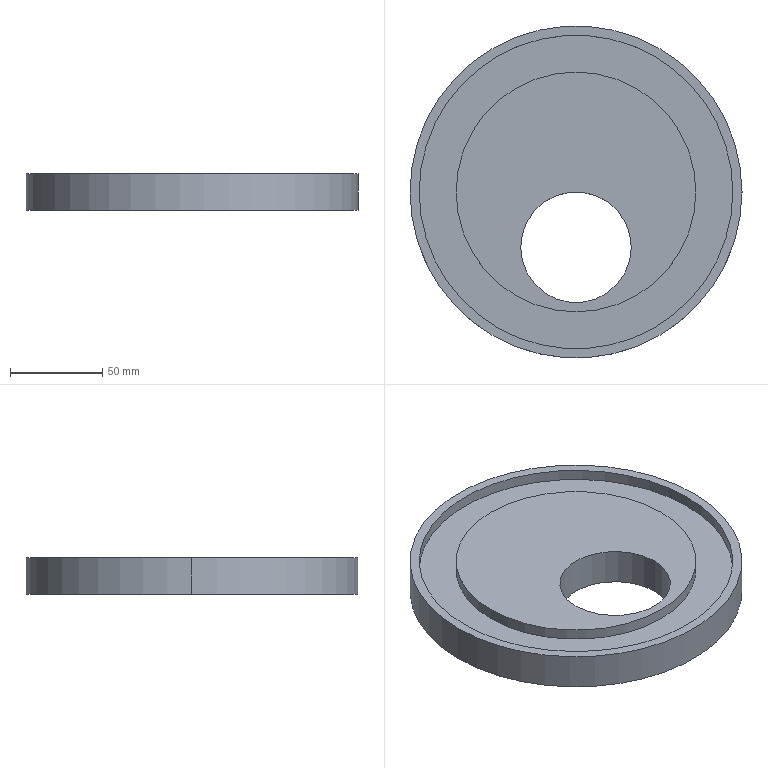Part | SolidWorks | features ICE 2, Extrusion 1 | 1 solid | 18 faces | box 180 x 180 x 20 mm | volume 339292 mm3 | cylinder 12 | plane 6 | commonest cylinder face diameters 130 x4 170 x4 60 x2 180 x2
STEP:
#1=CARTESIAN_POINT('',(-65.,30.,6.));
#2=VERTEX_POINT('',#1);
#3=CARTESIAN_POINT('',(65.,30.,6.));
#4=VERTEX_POINT('',#3);
#5=CARTESIAN_POINT('',(0.,30.,6.));
#6=DIRECTION('',(0.,0.,-1.));
#7=DIRECTION('',(-1.,0.,0.));
#8=AXIS2_PLACEMENT_3D('',#5,#6,#7);
#9=CIRCLE('',#8,65.);
#10=EDGE_CURVE('',#2,#4,#9,.T.);
#11=ORIENTED_EDGE('',*,*,#10,.T.);
#12=CARTESIAN_POINT('',(65.,30.,0.));
#13=VERTEX_POINT('',#12);
#14=CARTESIAN_POINT('',(65.,30.,6.));
#15=DIRECTION('',(0.,0.,-1.));
#16=VECTOR('',#15,1000.);
#17=LINE('',#14,#16);
#18=EDGE_CURVE('',#4,#13,#17,.T.);
#19=ORIENTED_EDGE('',*,*,#18,.T.);
#20=CARTESIAN_POINT('',(-65.,30.,0.));
#21=VERTEX_POINT('',#20);
#22=CARTESIAN_POINT('',(0.,30.,0.));
#23=DIRECTION('',(0.,0.,-1.));
#24=DIRECTION('',(-1.,0.,0.));
#25=AXIS2_PLACEMENT_3D('',#22,#23,#24);
#26=CIRCLE('',#25,65.);
#27=EDGE_CURVE('',#21,#13,#26,.T.);
#28=ORIENTED_EDGE('',*,*,#27,.F.);
#29=CARTESIAN_POINT('',(-65.,30.,6.));
#30=DIRECTION('',(0.,0.,-1.));
#31=VECTOR('',#30,1000.);
#32=LINE('',#29,#31);
#33=EDGE_CURVE('',#2,#21,#32,.T.);
#34=ORIENTED_EDGE('',*,*,#33,.F.);
#35=EDGE_LOOP('',(#11,#19,#28,#34));
#36=FACE_OUTER_BOUND('',#35,.T.);
#37=CARTESIAN_POINT('',(0.,30.,6.));
#38=DIRECTION('',(0.,0.,-1.));
#39=DIRECTION('',(-1.,0.,0.));
#40=AXIS2_PLACEMENT_3D('',#37,#38,#39);
#41=CYLINDRICAL_SURFACE('',#40,65.);
#42=ADVANCED_FACE('',(#36),#41,.T.);
#43=CARTESIAN_POINT('',(85.,30.,6.));
#44=VERTEX_POINT('',#43);
#45=CARTESIAN_POINT('',(-85.,30.,6.));
#46=VERTEX_POINT('',#45);
#47=CARTESIAN_POINT('',(0.,30.,6.));
#48=DIRECTION('',(0.,0.,-1.));
#49=DIRECTION('',(-1.,0.,0.));
#50=AXIS2_PLACEMENT_3D('',#47,#48,#49);
#51=CIRCLE('',#50,85.);
#52=EDGE_CURVE('',#44,#46,#51,.T.);
#53=ORIENTED_EDGE('',*,*,#52,.F.);
#54=CARTESIAN_POINT('',(85.,30.,0.));
#55=VERTEX_POINT('',#54);
#56=CARTESIAN_POINT('',(85.,30.,6.));
#57=DIRECTION('',(0.,0.,-1.));
#58=VECTOR('',#57,1000.);
#59=LINE('',#56,#58);
#60=EDGE_CURVE('',#44,#55,#59,.T.);
#61=ORIENTED_EDGE('',*,*,#60,.T.);
#62=CARTESIAN_POINT('',(-85.,30.,0.));
#63=VERTEX_POINT('',#62);
#64=CARTESIAN_POINT('',(0.,30.,0.));
#65=DIRECTION('',(0.,0.,-1.));
#66=DIRECTION('',(-1.,0.,0.));
#67=AXIS2_PLACEMENT_3D('',#64,#65,#66);
#68=CIRCLE('',#67,85.);
#69=EDGE_CURVE('',#55,#63,#68,.T.);
#70=ORIENTED_EDGE('',*,*,#69,.T.);
#71=CARTESIAN_POINT('',(-85.,30.,6.));
#72=DIRECTION('',(0.,0.,-1.));
#73=VECTOR('',#72,1000.);
#74=LINE('',#71,#73);
#75=EDGE_CURVE('',#46,#63,#74,.T.);
#76=ORIENTED_EDGE('',*,*,#75,.F.);
#77=EDGE_LOOP('',(#53,#61,#70,#76));
#78=FACE_OUTER_BOUND('',#77,.T.);
#79=CARTESIAN_POINT('',(0.,30.,6.));
#80=DIRECTION('',(0.,0.,-1.));
#81=DIRECTION('',(-1.,0.,0.));
#82=AXIS2_PLACEMENT_3D('',#79,#80,#81);
#83=CYLINDRICAL_SURFACE('',#82,85.);
#84=ADVANCED_FACE('',(#78),#83,.F.);
#85=CARTESIAN_POINT('',(65.,30.,14.));
#86=VERTEX_POINT('',#85);
#87=CARTESIAN_POINT('',(-65.,30.,14.));
#88=VERTEX_POINT('',#87);
#89=CARTESIAN_POINT('',(0.,30.,14.));
#90=DIRECTION('',(0.,0.,1.));
#91=DIRECTION('',(1.,0.,0.));
#92=AXIS2_PLACEMENT_3D('',#89,#90,#91);
#93=CIRCLE('',#92,65.);
#94=EDGE_CURVE('',#86,#88,#93,.T.);
#95=ORIENTED_EDGE('',*,*,#94,.T.);
#96=CARTESIAN_POINT('',(-65.,30.,20.));
#97=VERTEX_POINT('',#96);
#98=CARTESIAN_POINT('',(-65.,30.,14.));
#99=DIRECTION('',(0.,0.,1.));
#100=VECTOR('',#99,1000.);
#101=LINE('',#98,#100);
#102=EDGE_CURVE('',#88,#97,#101,.T.);
#103=ORIENTED_EDGE('',*,*,#102,.T.);
#104=CARTESIAN_POINT('',(65.,30.,20.));
#105=VERTEX_POINT('',#104);
#106=CARTESIAN_POINT('',(0.,30.,20.));
#107=DIRECTION('',(0.,0.,1.));
#108=DIRECTION('',(1.,0.,0.));
#109=AXIS2_PLACEMENT_3D('',#106,#107,#108);
#110=CIRCLE('',#109,65.);
#111=EDGE_CURVE('',#105,#97,#110,.T.);
#112=ORIENTED_EDGE('',*,*,#111,.F.);
#113=CARTESIAN_POINT('',(65.,30.,14.));
#114=DIRECTION('',(0.,0.,1.));
#115=VECTOR('',#114,1000.);
#116=LINE('',#113,#115);
#117=EDGE_CURVE('',#86,#105,#116,.T.);
#118=ORIENTED_EDGE('',*,*,#117,.F.);
#119=EDGE_LOOP('',(#95,#103,#112,#118));
#120=FACE_OUTER_BOUND('',#119,.T.);
#121=CARTESIAN_POINT('',(0.,30.,14.));
#122=DIRECTION('',(0.,0.,1.));
#123=DIRECTION('',(1.,0.,0.));
#124=AXIS2_PLACEMENT_3D('',#121,#122,#123);
#125=CYLINDRICAL_SURFACE('',#124,65.);
#126=ADVANCED_FACE('',(#120),#125,.T.);
#127=CARTESIAN_POINT('',(-85.,30.,14.));
#128=VERTEX_POINT('',#127);
#129=CARTESIAN_POINT('',(85.,30.,14.));
#130=VERTEX_POINT('',#129);
#131=CARTESIAN_POINT('',(0.,30.,14.));
#132=DIRECTION('',(0.,0.,1.));
#133=DIRECTION('',(1.,0.,0.));
#134=AXIS2_PLACEMENT_3D('',#131,#132,#133);
#135=CIRCLE('',#134,85.);
#136=EDGE_CURVE('',#128,#130,#135,.T.);
#137=ORIENTED_EDGE('',*,*,#136,.F.);
#138=CARTESIAN_POINT('',(-85.,30.,20.));
#139=VERTEX_POINT('',#138);
#140=CARTESIAN_POINT('',(-85.,30.,14.));
#141=DIRECTION('',(0.,0.,1.));
#142=VECTOR('',#141,1000.);
#143=LINE('',#140,#142);
#144=EDGE_CURVE('',#128,#139,#143,.T.);
#145=ORIENTED_EDGE('',*,*,#144,.T.);
#146=CARTESIAN_POINT('',(85.,30.,20.));
#147=VERTEX_POINT('',#146);
#148=CARTESIAN_POINT('',(0.,30.,20.));
#149=DIRECTION('',(0.,0.,1.));
#150=DIRECTION('',(1.,0.,0.));
#151=AXIS2_PLACEMENT_3D('',#148,#149,#150);
#152=CIRCLE('',#151,85.);
#153=EDGE_CURVE('',#139,#147,#152,.T.);
#154=ORIENTED_EDGE('',*,*,#153,.T.);
#155=CARTESIAN_POINT('',(85.,30.,14.));
#156=DIRECTION('',(0.,0.,1.));
#157=VECTOR('',#156,1000.);
#158=LINE('',#155,#157);
#159=EDGE_CURVE('',#130,#147,#158,.T.);
#160=ORIENTED_EDGE('',*,*,#159,.F.);
#161=EDGE_LOOP('',(#137,#145,#154,#160));
#162=FACE_OUTER_BOUND('',#161,.T.);
#163=CARTESIAN_POINT('',(0.,30.,14.));
#164=DIRECTION('',(0.,0.,1.));
#165=DIRECTION('',(1.,0.,0.));
#166=AXIS2_PLACEMENT_3D('',#163,#164,#165);
#167=CYLINDRICAL_SURFACE('',#166,85.);
#168=ADVANCED_FACE('',(#162),#167,.F.);
#169=CARTESIAN_POINT('',(-30.,0.,20.));
#170=VERTEX_POINT('',#169);
#171=CARTESIAN_POINT('',(30.,0.,20.));
#172=VERTEX_POINT('',#171);
#173=CARTESIAN_POINT('',(0.,0.,20.));
#174=DIRECTION('',(0.,0.,1.));
#175=DIRECTION('',(1.,0.,0.));
#176=AXIS2_PLACEMENT_3D('',#173,#174,#175);
#177=CIRCLE('',#176,30.);
#178=EDGE_CURVE('',#170,#172,#177,.T.);
#179=ORIENTED_EDGE('',*,*,#178,.T.);
#180=CARTESIAN_POINT('',(30.,0.,0.));
#181=VERTEX_POINT('',#180);
#182=CARTESIAN_POINT('',(30.,0.,20.));
#183=DIRECTION('',(0.,0.,-1.));
#184=VECTOR('',#183,1000.);
#185=LINE('',#182,#184);
#186=EDGE_CURVE('',#172,#181,#185,.T.);
#187=ORIENTED_EDGE('',*,*,#186,.T.);
#188=CARTESIAN_POINT('',(-30.,0.,0.));
#189=VERTEX_POINT('',#188);
#190=CARTESIAN_POINT('',(0.,0.,0.));
#191=DIRECTION('',(0.,0.,1.));
#192=DIRECTION('',(1.,0.,0.));
#193=AXIS2_PLACEMENT_3D('',#190,#191,#192);
#194=CIRCLE('',#193,30.);
#195=EDGE_CURVE('',#189,#181,#194,.T.);
#196=ORIENTED_EDGE('',*,*,#195,.F.);
#197=CARTESIAN_POINT('',(-30.,0.,20.));
#198=DIRECTION('',(0.,0.,-1.));
#199=VECTOR('',#198,1000.);
#200=LINE('',#197,#199);
#201=EDGE_CURVE('',#170,#189,#200,.T.);
#202=ORIENTED_EDGE('',*,*,#201,.F.);
#203=EDGE_LOOP('',(#179,#187,#196,#202));
#204=FACE_OUTER_BOUND('',#203,.T.);
#205=CARTESIAN_POINT('',(0.,0.,20.));
#206=DIRECTION('',(0.,0.,-1.));
#207=DIRECTION('',(-1.,0.,0.));
#208=AXIS2_PLACEMENT_3D('',#205,#206,#207);
#209=CYLINDRICAL_SURFACE('',#208,30.);
#210=ADVANCED_FACE('',(#204),#209,.F.);
#211=CARTESIAN_POINT('',(90.,30.,20.));
#212=VERTEX_POINT('',#211);
#213=CARTESIAN_POINT('',(-90.,30.,20.));
#214=VERTEX_POINT('',#213);
#215=CARTESIAN_POINT('',(0.,30.,20.));
#216=DIRECTION('',(0.,0.,1.));
#217=DIRECTION('',(1.,0.,0.));
#218=AXIS2_PLACEMENT_3D('',#215,#216,#217);
#219=CIRCLE('',#218,90.);
#220=EDGE_CURVE('',#212,#214,#219,.T.);
#221=ORIENTED_EDGE('',*,*,#220,.F.);
#222=CARTESIAN_POINT('',(90.,30.,0.));
#223=VERTEX_POINT('',#222);
#224=CARTESIAN_POINT('',(90.,30.,20.));
#225=DIRECTION('',(0.,0.,-1.));
#226=VECTOR('',#225,1000.);
#227=LINE('',#224,#226);
#228=EDGE_CURVE('',#212,#223,#227,.T.);
#229=ORIENTED_EDGE('',*,*,#228,.T.);
#230=CARTESIAN_POINT('',(-90.,30.,0.));
#231=VERTEX_POINT('',#230);
#232=CARTESIAN_POINT('',(0.,30.,0.));
#233=DIRECTION('',(0.,0.,1.));
#234=DIRECTION('',(1.,0.,0.));
#235=AXIS2_PLACEMENT_3D('',#232,#233,#234);
#236=CIRCLE('',#235,90.);
#237=EDGE_CURVE('',#223,#231,#236,.T.);
#238=ORIENTED_EDGE('',*,*,#237,.T.);
#239=CARTESIAN_POINT('',(-90.,30.,20.));
#240=DIRECTION('',(0.,0.,-1.));
#241=VECTOR('',#240,1000.);
#242=LINE('',#239,#241);
#243=EDGE_CURVE('',#214,#231,#242,.T.);
#244=ORIENTED_EDGE('',*,*,#243,.F.);
#245=EDGE_LOOP('',(#221,#229,#238,#244));
#246=FACE_OUTER_BOUND('',#245,.T.);
#247=CARTESIAN_POINT('',(0.,30.,20.));
#248=DIRECTION('',(0.,0.,-1.));
#249=DIRECTION('',(-1.,0.,0.));
#250=AXIS2_PLACEMENT_3D('',#247,#248,#249);
#251=CYLINDRICAL_SURFACE('',#250,90.);
#252=ADVANCED_FACE('',(#246),#251,.T.);
#253=ORIENTED_EDGE('',*,*,#195,.T.);
#254=CARTESIAN_POINT('',(0.,0.,0.));
#255=DIRECTION('',(0.,0.,1.));
#256=DIRECTION('',(1.,0.,0.));
#257=AXIS2_PLACEMENT_3D('',#254,#255,#256);
#258=CIRCLE('',#257,30.);
#259=EDGE_CURVE('',#181,#189,#258,.T.);
#260=ORIENTED_EDGE('',*,*,#259,.T.);
#261=EDGE_LOOP('',(#253,#260));
#262=FACE_BOUND('',#261,.T.);
#263=ORIENTED_EDGE('',*,*,#27,.T.);
#264=CARTESIAN_POINT('',(0.,30.,0.));
#265=DIRECTION('',(0.,0.,-1.));
#266=DIRECTION('',(-1.,0.,0.));
#267=AXIS2_PLACEMENT_3D('',#264,#265,#266);
#268=CIRCLE('',#267,65.);
#269=EDGE_CURVE('',#13,#21,#268,.T.);
#270=ORIENTED_EDGE('',*,*,#269,.T.);
#271=EDGE_LOOP('',(#263,#270));
#272=FACE_OUTER_BOUND('',#271,.T.);
#273=CARTESIAN_POINT('',(0.,30.,0.));
#274=DIRECTION('',(0.,0.,1.));
#275=DIRECTION('',(1.,0.,0.));
#276=AXIS2_PLACEMENT_3D('',#273,#274,#275);
#277=PLANE('',#276);
#278=ADVANCED_FACE('',(#262,#272),#277,.F.);
#279=ORIENTED_EDGE('',*,*,#178,.F.);
#280=CARTESIAN_POINT('',(0.,0.,20.));
#281=DIRECTION('',(0.,0.,1.));
#282=DIRECTION('',(1.,0.,0.));
#283=AXIS2_PLACEMENT_3D('',#280,#281,#282);
#284=CIRCLE('',#283,30.);
#285=EDGE_CURVE('',#172,#170,#284,.T.);
#286=ORIENTED_EDGE('',*,*,#285,.F.);
#287=EDGE_LOOP('',(#279,#286));
#288=FACE_BOUND('',#287,.T.);
#289=ORIENTED_EDGE('',*,*,#111,.T.);
#290=CARTESIAN_POINT('',(0.,30.,20.));
#291=DIRECTION('',(0.,0.,1.));
#292=DIRECTION('',(1.,0.,0.));
#293=AXIS2_PLACEMENT_3D('',#290,#291,#292);
#294=CIRCLE('',#293,65.);
#295=EDGE_CURVE('',#97,#105,#294,.T.);
#296=ORIENTED_EDGE('',*,*,#295,.T.);
#297=EDGE_LOOP('',(#289,#296));
#298=FACE_OUTER_BOUND('',#297,.T.);
#299=CARTESIAN_POINT('',(0.,30.,20.));
#300=DIRECTION('',(0.,0.,1.));
#301=DIRECTION('',(1.,0.,0.));
#302=AXIS2_PLACEMENT_3D('',#299,#300,#301);
#303=PLANE('',#302);
#304=ADVANCED_FACE('',(#288,#298),#303,.T.);
#305=CARTESIAN_POINT('',(0.,30.,20.));
#306=DIRECTION('',(0.,0.,1.));
#307=DIRECTION('',(1.,0.,0.));
#308=AXIS2_PLACEMENT_3D('',#305,#306,#307);
#309=CIRCLE('',#308,85.);
#310=EDGE_CURVE('',#147,#139,#309,.T.);
#311=ORIENTED_EDGE('',*,*,#310,.F.);
#312=ORIENTED_EDGE('',*,*,#153,.F.);
#313=EDGE_LOOP('',(#311,#312));
#314=FACE_BOUND('',#313,.T.);
#315=CARTESIAN_POINT('',(0.,30.,20.));
#316=DIRECTION('',(0.,0.,1.));
#317=DIRECTION('',(1.,0.,0.));
#318=AXIS2_PLACEMENT_3D('',#315,#316,#317);
#319=CIRCLE('',#318,90.);
#320=EDGE_CURVE('',#214,#212,#319,.T.);
#321=ORIENTED_EDGE('',*,*,#320,.T.);
#322=ORIENTED_EDGE('',*,*,#220,.T.);
#323=EDGE_LOOP('',(#321,#322));
#324=FACE_OUTER_BOUND('',#323,.T.);
#325=CARTESIAN_POINT('',(0.,30.,20.));
#326=DIRECTION('',(0.,0.,1.));
#327=DIRECTION('',(1.,0.,0.));
#328=AXIS2_PLACEMENT_3D('',#325,#326,#327);
#329=PLANE('',#328);
#330=ADVANCED_FACE('',(#314,#324),#329,.T.);
#331=CARTESIAN_POINT('',(0.,30.,0.));
#332=DIRECTION('',(0.,0.,-1.));
#333=DIRECTION('',(-1.,0.,0.));
#334=AXIS2_PLACEMENT_3D('',#331,#332,#333);
#335=CIRCLE('',#334,85.);
#336=EDGE_CURVE('',#63,#55,#335,.T.);
#337=ORIENTED_EDGE('',*,*,#336,.F.);
#338=ORIENTED_EDGE('',*,*,#69,.F.);
#339=EDGE_LOOP('',(#337,#338));
#340=FACE_BOUND('',#339,.T.);
#341=CARTESIAN_POINT('',(0.,30.,0.));
#342=DIRECTION('',(0.,0.,1.));
#343=DIRECTION('',(1.,0.,0.));
#344=AXIS2_PLACEMENT_3D('',#341,#342,#343);
#345=CIRCLE('',#344,90.);
#346=EDGE_CURVE('',#231,#223,#345,.T.);
#347=ORIENTED_EDGE('',*,*,#346,.F.);
#348=ORIENTED_EDGE('',*,*,#237,.F.);
#349=EDGE_LOOP('',(#347,#348));
#350=FACE_OUTER_BOUND('',#349,.T.);
#351=CARTESIAN_POINT('',(0.,30.,0.));
#352=DIRECTION('',(0.,0.,1.));
#353=DIRECTION('',(1.,0.,0.));
#354=AXIS2_PLACEMENT_3D('',#351,#352,#353);
#355=PLANE('',#354);
#356=ADVANCED_FACE('',(#340,#350),#355,.F.);
#357=ORIENTED_EDGE('',*,*,#228,.F.);
#358=ORIENTED_EDGE('',*,*,#320,.F.);
#359=ORIENTED_EDGE('',*,*,#243,.T.);
#360=ORIENTED_EDGE('',*,*,#346,.T.);
#361=EDGE_LOOP('',(#357,#358,#359,#360));
#362=FACE_OUTER_BOUND('',#361,.T.);
#363=CARTESIAN_POINT('',(0.,30.,20.));
#364=DIRECTION('',(0.,0.,-1.));
#365=DIRECTION('',(-1.,0.,0.));
#366=AXIS2_PLACEMENT_3D('',#363,#364,#365);
#367=CYLINDRICAL_SURFACE('',#366,90.);
#368=ADVANCED_FACE('',(#362),#367,.T.);
#369=ORIENTED_EDGE('',*,*,#186,.F.);
#370=ORIENTED_EDGE('',*,*,#285,.T.);
#371=ORIENTED_EDGE('',*,*,#201,.T.);
#372=ORIENTED_EDGE('',*,*,#259,.F.);
#373=EDGE_LOOP('',(#369,#370,#371,#372));
#374=FACE_OUTER_BOUND('',#373,.T.);
#375=CARTESIAN_POINT('',(0.,0.,20.));
#376=DIRECTION('',(0.,0.,-1.));
#377=DIRECTION('',(-1.,0.,0.));
#378=AXIS2_PLACEMENT_3D('',#375,#376,#377);
#379=CYLINDRICAL_SURFACE('',#378,30.);
#380=ADVANCED_FACE('',(#374),#379,.F.);
#381=ORIENTED_EDGE('',*,*,#144,.F.);
#382=CARTESIAN_POINT('',(0.,30.,14.));
#383=DIRECTION('',(0.,0.,1.));
#384=DIRECTION('',(1.,0.,0.));
#385=AXIS2_PLACEMENT_3D('',#382,#383,#384);
#386=CIRCLE('',#385,85.);
#387=EDGE_CURVE('',#130,#128,#386,.T.);
#388=ORIENTED_EDGE('',*,*,#387,.F.);
#389=ORIENTED_EDGE('',*,*,#159,.T.);
#390=ORIENTED_EDGE('',*,*,#310,.T.);
#391=EDGE_LOOP('',(#381,#388,#389,#390));
#392=FACE_OUTER_BOUND('',#391,.T.);
#393=CARTESIAN_POINT('',(0.,30.,14.));
#394=DIRECTION('',(0.,0.,1.));
#395=DIRECTION('',(1.,0.,0.));
#396=AXIS2_PLACEMENT_3D('',#393,#394,#395);
#397=CYLINDRICAL_SURFACE('',#396,85.);
#398=ADVANCED_FACE('',(#392),#397,.F.);
#399=ORIENTED_EDGE('',*,*,#94,.F.);
#400=CARTESIAN_POINT('',(0.,30.,14.));
#401=DIRECTION('',(0.,0.,1.));
#402=DIRECTION('',(1.,0.,0.));
#403=AXIS2_PLACEMENT_3D('',#400,#401,#402);
#404=CIRCLE('',#403,65.);
#405=EDGE_CURVE('',#88,#86,#404,.T.);
#406=ORIENTED_EDGE('',*,*,#405,.F.);
#407=EDGE_LOOP('',(#399,#406));
#408=FACE_BOUND('',#407,.T.);
#409=ORIENTED_EDGE('',*,*,#387,.T.);
#410=ORIENTED_EDGE('',*,*,#136,.T.);
#411=EDGE_LOOP('',(#409,#410));
#412=FACE_OUTER_BOUND('',#411,.T.);
#413=CARTESIAN_POINT('',(0.,30.,14.));
#414=DIRECTION('',(0.,0.,1.));
#415=DIRECTION('',(1.,0.,0.));
#416=AXIS2_PLACEMENT_3D('',#413,#414,#415);
#417=PLANE('',#416);
#418=ADVANCED_FACE('',(#408,#412),#417,.T.);
#419=ORIENTED_EDGE('',*,*,#102,.F.);
#420=ORIENTED_EDGE('',*,*,#405,.T.);
#421=ORIENTED_EDGE('',*,*,#117,.T.);
#422=ORIENTED_EDGE('',*,*,#295,.F.);
#423=EDGE_LOOP('',(#419,#420,#421,#422));
#424=FACE_OUTER_BOUND('',#423,.T.);
#425=CARTESIAN_POINT('',(0.,30.,14.));
#426=DIRECTION('',(0.,0.,1.));
#427=DIRECTION('',(1.,0.,0.));
#428=AXIS2_PLACEMENT_3D('',#425,#426,#427);
#429=CYLINDRICAL_SURFACE('',#428,65.);
#430=ADVANCED_FACE('',(#424),#429,.T.);
#431=ORIENTED_EDGE('',*,*,#60,.F.);
#432=CARTESIAN_POINT('',(0.,30.,6.));
#433=DIRECTION('',(0.,0.,-1.));
#434=DIRECTION('',(-1.,0.,0.));
#435=AXIS2_PLACEMENT_3D('',#432,#433,#434);
#436=CIRCLE('',#435,85.);
#437=EDGE_CURVE('',#46,#44,#436,.T.);
#438=ORIENTED_EDGE('',*,*,#437,.F.);
#439=ORIENTED_EDGE('',*,*,#75,.T.);
#440=ORIENTED_EDGE('',*,*,#336,.T.);
#441=EDGE_LOOP('',(#431,#438,#439,#440));
#442=FACE_OUTER_BOUND('',#441,.T.);
#443=CARTESIAN_POINT('',(0.,30.,6.));
#444=DIRECTION('',(0.,0.,-1.));
#445=DIRECTION('',(-1.,0.,0.));
#446=AXIS2_PLACEMENT_3D('',#443,#444,#445);
#447=CYLINDRICAL_SURFACE('',#446,85.);
#448=ADVANCED_FACE('',(#442),#447,.F.);
#449=ORIENTED_EDGE('',*,*,#10,.F.);
#450=CARTESIAN_POINT('',(0.,30.,6.));
#451=DIRECTION('',(0.,0.,-1.));
#452=DIRECTION('',(-1.,0.,0.));
#453=AXIS2_PLACEMENT_3D('',#450,#451,#452);
#454=CIRCLE('',#453,65.);
#455=EDGE_CURVE('',#4,#2,#454,.T.);
#456=ORIENTED_EDGE('',*,*,#455,.F.);
#457=EDGE_LOOP('',(#449,#456));
#458=FACE_BOUND('',#457,.T.);
#459=ORIENTED_EDGE('',*,*,#437,.T.);
#460=ORIENTED_EDGE('',*,*,#52,.T.);
#461=EDGE_LOOP('',(#459,#460));
#462=FACE_OUTER_BOUND('',#461,.T.);
#463=CARTESIAN_POINT('',(0.,30.,6.));
#464=DIRECTION('',(0.,0.,-1.));
#465=DIRECTION('',(-1.,0.,0.));
#466=AXIS2_PLACEMENT_3D('',#463,#464,#465);
#467=PLANE('',#466);
#468=ADVANCED_FACE('',(#458,#462),#467,.T.);
#469=ORIENTED_EDGE('',*,*,#18,.F.);
#470=ORIENTED_EDGE('',*,*,#455,.T.);
#471=ORIENTED_EDGE('',*,*,#33,.T.);
#472=ORIENTED_EDGE('',*,*,#269,.F.);
#473=EDGE_LOOP('',(#469,#470,#471,#472));
#474=FACE_OUTER_BOUND('',#473,.T.);
#475=CARTESIAN_POINT('',(0.,30.,6.));
#476=DIRECTION('',(0.,0.,-1.));
#477=DIRECTION('',(-1.,0.,0.));
#478=AXIS2_PLACEMENT_3D('',#475,#476,#477);
#479=CYLINDRICAL_SURFACE('',#478,65.);
#480=ADVANCED_FACE('',(#474),#479,.T.);
#481=CLOSED_SHELL('',(#42,#84,#126,#168,#210,#252,#278,#304,#330,#356,#368,#380,#398,#418,#430,#448,#468,#480));
#482=MANIFOLD_SOLID_BREP('',#481);
#483=CARTESIAN_POINT('',(0.,0.,0.));
#484=DIRECTION('',(0.,0.,1.));
#485=DIRECTION('',(1.,0.,0.));
#486=AXIS2_PLACEMENT_3D('',#483,#484,#485);
#487=(LENGTH_UNIT()NAMED_UNIT(*)SI_UNIT(.MILLI.,.METRE.));
#488=UNCERTAINTY_MEASURE_WITH_UNIT(LENGTH_MEASURE(0.00001),#487,'','');
#489=(NAMED_UNIT(*)PLANE_ANGLE_UNIT()SI_UNIT($,.RADIAN.));
#490=(NAMED_UNIT(*)SI_UNIT($,.STERADIAN.)SOLID_ANGLE_UNIT());
#491=(GEOMETRIC_REPRESENTATION_CONTEXT(3)GLOBAL_UNCERTAINTY_ASSIGNED_CONTEXT((#488))GLOBAL_UNIT_ASSIGNED_CONTEXT((#487,#489,#490))REPRESENTATION_CONTEXT('',''));
#492=ADVANCED_BREP_SHAPE_REPRESENTATION('',(#482,#486),#491);